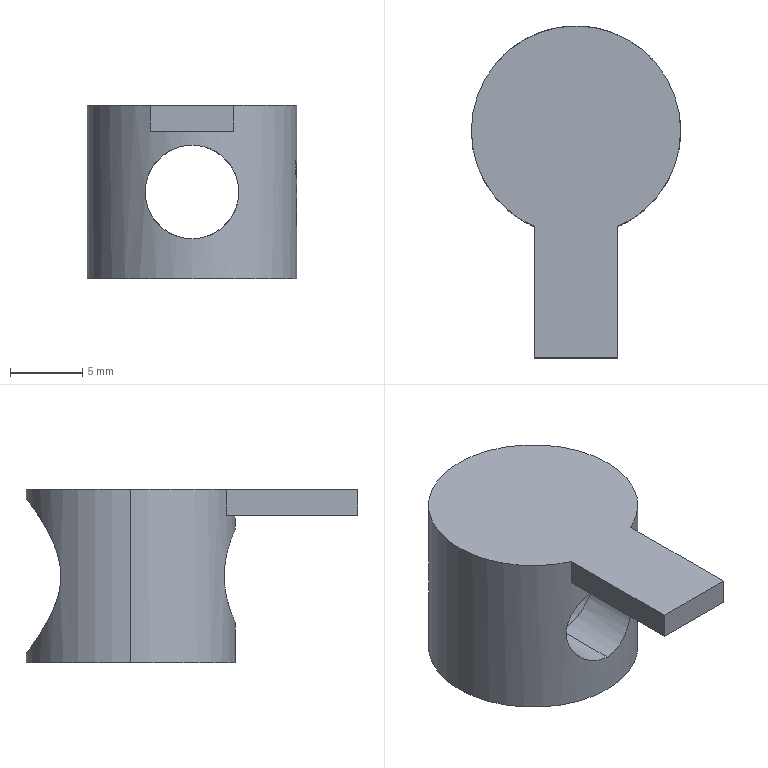Part | NX | features BREP 1 | 1 solid | 55 faces | box 14.5 x 23 x 12 mm | volume 1063 mm3 | plane 33 | cylinder 13 | spline 9 | commonest cylinder face diameters 14.5 x9 6.5 x2 10.8 x2